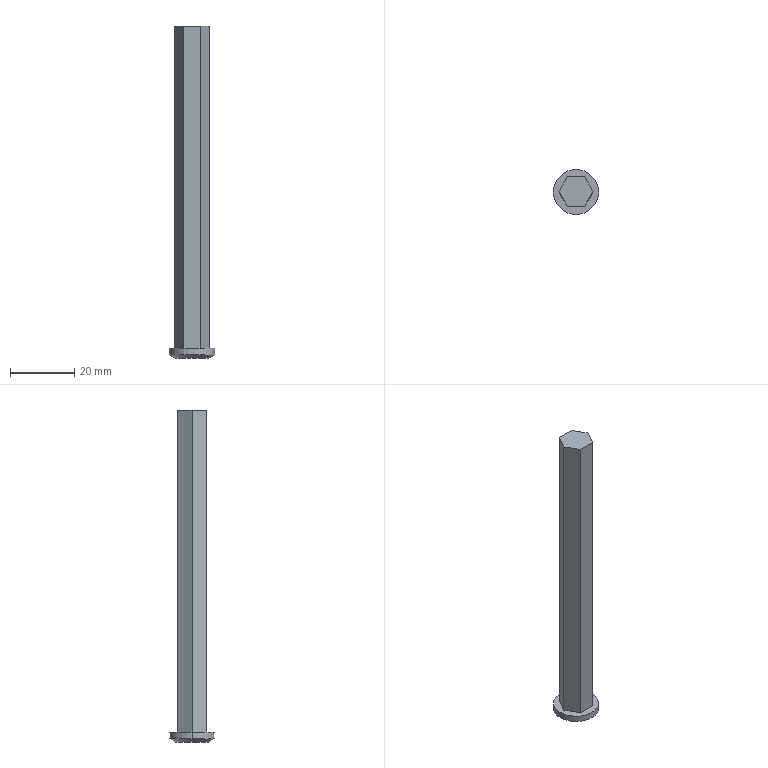Part | SolidWorks | features Chamfer 1, Extrusion 1, ICE 1 | 1 solid | 13 faces | box 14 x 14 x 103 mm | volume 7725 mm3 | plane 9 | cone 2 | cylinder 2 | commonest cylinder face diameters 14 x2
STEP:
#1=CARTESIAN_POINT('',(-5.268,0.,-3.));
#2=VERTEX_POINT('',#1);
#3=CARTESIAN_POINT('',(5.268,0.,-3.));
#4=VERTEX_POINT('',#3);
#5=CARTESIAN_POINT('',(0.,0.,-3.));
#6=DIRECTION('',(0.,0.,-1.));
#7=DIRECTION('',(-1.,0.,0.));
#8=AXIS2_PLACEMENT_3D('',#5,#6,#7);
#9=CIRCLE('',#8,5.268);
#10=EDGE_CURVE('',#2,#4,#9,.T.);
#11=ORIENTED_EDGE('',*,*,#10,.F.);
#12=CARTESIAN_POINT('',(-7.,0.,-2.));
#13=VERTEX_POINT('',#12);
#14=CARTESIAN_POINT('',(-5.268,0.,-3.));
#15=DIRECTION('',(-0.866,0.,0.5));
#16=VECTOR('',#15,1000.);
#17=LINE('',#14,#16);
#18=EDGE_CURVE('',#2,#13,#17,.T.);
#19=ORIENTED_EDGE('',*,*,#18,.T.);
#20=CARTESIAN_POINT('',(7.,0.,-2.));
#21=VERTEX_POINT('',#20);
#22=CARTESIAN_POINT('',(0.,0.,-2.));
#23=DIRECTION('',(0.,0.,1.));
#24=DIRECTION('',(-1.,0.,0.));
#25=AXIS2_PLACEMENT_3D('',#22,#23,#24);
#26=CIRCLE('',#25,7.);
#27=EDGE_CURVE('',#21,#13,#26,.T.);
#28=ORIENTED_EDGE('',*,*,#27,.F.);
#29=CARTESIAN_POINT('',(5.268,0.,-3.));
#30=DIRECTION('',(0.866,0.,0.5));
#31=VECTOR('',#30,1000.);
#32=LINE('',#29,#31);
#33=EDGE_CURVE('',#4,#21,#32,.T.);
#34=ORIENTED_EDGE('',*,*,#33,.F.);
#35=EDGE_LOOP('',(#11,#19,#28,#34));
#36=FACE_OUTER_BOUND('',#35,.T.);
#37=CARTESIAN_POINT('',(0.,0.,-3.));
#38=DIRECTION('',(0.,0.,1.));
#39=DIRECTION('',(1.,0.,0.));
#40=AXIS2_PLACEMENT_3D('',#37,#38,#39);
#41=CONICAL_SURFACE('',#40,5.268,1.047);
#42=ADVANCED_FACE('',(#36),#41,.T.);
#43=ORIENTED_EDGE('',*,*,#27,.T.);
#44=CARTESIAN_POINT('',(-7.,0.,0.));
#45=VERTEX_POINT('',#44);
#46=CARTESIAN_POINT('',(-7.,0.,-3.));
#47=DIRECTION('',(0.,0.,1.));
#48=VECTOR('',#47,1000.);
#49=LINE('',#46,#48);
#50=EDGE_CURVE('',#13,#45,#49,.T.);
#51=ORIENTED_EDGE('',*,*,#50,.T.);
#52=CARTESIAN_POINT('',(7.,0.,0.));
#53=VERTEX_POINT('',#52);
#54=CARTESIAN_POINT('',(0.,0.,0.));
#55=DIRECTION('',(0.,0.,-1.));
#56=DIRECTION('',(-1.,0.,0.));
#57=AXIS2_PLACEMENT_3D('',#54,#55,#56);
#58=CIRCLE('',#57,7.);
#59=EDGE_CURVE('',#45,#53,#58,.T.);
#60=ORIENTED_EDGE('',*,*,#59,.T.);
#61=CARTESIAN_POINT('',(7.,0.,-3.));
#62=DIRECTION('',(0.,0.,1.));
#63=VECTOR('',#62,1000.);
#64=LINE('',#61,#63);
#65=EDGE_CURVE('',#21,#53,#64,.T.);
#66=ORIENTED_EDGE('',*,*,#65,.F.);
#67=EDGE_LOOP('',(#43,#51,#60,#66));
#68=FACE_OUTER_BOUND('',#67,.T.);
#69=CARTESIAN_POINT('',(0.,0.,-3.));
#70=DIRECTION('',(0.,0.,1.));
#71=DIRECTION('',(1.,0.,0.));
#72=AXIS2_PLACEMENT_3D('',#69,#70,#71);
#73=CYLINDRICAL_SURFACE('',#72,7.);
#74=ADVANCED_FACE('',(#68),#73,.T.);
#75=CARTESIAN_POINT('',(-2.65,-4.59,0.));
#76=VERTEX_POINT('',#75);
#77=CARTESIAN_POINT('',(2.65,-4.59,0.));
#78=VERTEX_POINT('',#77);
#79=CARTESIAN_POINT('',(-2.65,-4.59,0.));
#80=DIRECTION('',(1.,0.,0.));
#81=VECTOR('',#80,1000.);
#82=LINE('',#79,#81);
#83=EDGE_CURVE('',#76,#78,#82,.T.);
#84=ORIENTED_EDGE('',*,*,#83,.T.);
#85=CARTESIAN_POINT('',(2.65,-4.59,100.));
#86=VERTEX_POINT('',#85);
#87=CARTESIAN_POINT('',(2.65,-4.59,100.));
#88=DIRECTION('',(0.,0.,-1.));
#89=VECTOR('',#88,1000.);
#90=LINE('',#87,#89);
#91=EDGE_CURVE('',#86,#78,#90,.T.);
#92=ORIENTED_EDGE('',*,*,#91,.F.);
#93=CARTESIAN_POINT('',(-2.65,-4.59,100.));
#94=VERTEX_POINT('',#93);
#95=CARTESIAN_POINT('',(-2.65,-4.59,100.));
#96=DIRECTION('',(1.,0.,0.));
#97=VECTOR('',#96,1000.);
#98=LINE('',#95,#97);
#99=EDGE_CURVE('',#94,#86,#98,.T.);
#100=ORIENTED_EDGE('',*,*,#99,.F.);
#101=CARTESIAN_POINT('',(-2.65,-4.59,100.));
#102=DIRECTION('',(0.,0.,-1.));
#103=VECTOR('',#102,1000.);
#104=LINE('',#101,#103);
#105=EDGE_CURVE('',#94,#76,#104,.T.);
#106=ORIENTED_EDGE('',*,*,#105,.T.);
#107=EDGE_LOOP('',(#84,#92,#100,#106));
#108=FACE_OUTER_BOUND('',#107,.T.);
#109=CARTESIAN_POINT('',(-2.65,-4.59,100.));
#110=DIRECTION('',(0.,1.,0.));
#111=DIRECTION('',(0.,0.,1.));
#112=AXIS2_PLACEMENT_3D('',#109,#110,#111);
#113=PLANE('',#112);
#114=ADVANCED_FACE('',(#108),#113,.F.);
#115=CARTESIAN_POINT('',(5.3,0.,0.));
#116=VERTEX_POINT('',#115);
#117=CARTESIAN_POINT('',(2.65,-4.59,0.));
#118=DIRECTION('',(0.5,0.866,0.));
#119=VECTOR('',#118,1000.);
#120=LINE('',#117,#119);
#121=EDGE_CURVE('',#78,#116,#120,.T.);
#122=ORIENTED_EDGE('',*,*,#121,.T.);
#123=CARTESIAN_POINT('',(5.3,0.,100.));
#124=VERTEX_POINT('',#123);
#125=CARTESIAN_POINT('',(5.3,0.,100.));
#126=DIRECTION('',(0.,0.,-1.));
#127=VECTOR('',#126,1000.);
#128=LINE('',#125,#127);
#129=EDGE_CURVE('',#124,#116,#128,.T.);
#130=ORIENTED_EDGE('',*,*,#129,.F.);
#131=CARTESIAN_POINT('',(2.65,-4.59,100.));
#132=DIRECTION('',(0.5,0.866,0.));
#133=VECTOR('',#132,1000.);
#134=LINE('',#131,#133);
#135=EDGE_CURVE('',#86,#124,#134,.T.);
#136=ORIENTED_EDGE('',*,*,#135,.F.);
#137=ORIENTED_EDGE('',*,*,#91,.T.);
#138=EDGE_LOOP('',(#122,#130,#136,#137));
#139=FACE_OUTER_BOUND('',#138,.T.);
#140=CARTESIAN_POINT('',(2.65,-4.59,100.));
#141=DIRECTION('',(-0.866,0.5,0.));
#142=DIRECTION('',(-0.5,-0.866,0.));
#143=AXIS2_PLACEMENT_3D('',#140,#141,#142);
#144=PLANE('',#143);
#145=ADVANCED_FACE('',(#139),#144,.F.);
#146=CARTESIAN_POINT('',(2.65,4.59,0.));
#147=VERTEX_POINT('',#146);
#148=CARTESIAN_POINT('',(5.3,0.,0.));
#149=DIRECTION('',(-0.5,0.866,0.));
#150=VECTOR('',#149,1000.);
#151=LINE('',#148,#150);
#152=EDGE_CURVE('',#116,#147,#151,.T.);
#153=ORIENTED_EDGE('',*,*,#152,.T.);
#154=CARTESIAN_POINT('',(2.65,4.59,100.));
#155=VERTEX_POINT('',#154);
#156=CARTESIAN_POINT('',(2.65,4.59,100.));
#157=DIRECTION('',(0.,0.,-1.));
#158=VECTOR('',#157,1000.);
#159=LINE('',#156,#158);
#160=EDGE_CURVE('',#155,#147,#159,.T.);
#161=ORIENTED_EDGE('',*,*,#160,.F.);
#162=CARTESIAN_POINT('',(5.3,0.,100.));
#163=DIRECTION('',(-0.5,0.866,0.));
#164=VECTOR('',#163,1000.);
#165=LINE('',#162,#164);
#166=EDGE_CURVE('',#124,#155,#165,.T.);
#167=ORIENTED_EDGE('',*,*,#166,.F.);
#168=ORIENTED_EDGE('',*,*,#129,.T.);
#169=EDGE_LOOP('',(#153,#161,#167,#168));
#170=FACE_OUTER_BOUND('',#169,.T.);
#171=CARTESIAN_POINT('',(5.3,0.,100.));
#172=DIRECTION('',(-0.866,-0.5,0.));
#173=DIRECTION('',(0.5,-0.866,0.));
#174=AXIS2_PLACEMENT_3D('',#171,#172,#173);
#175=PLANE('',#174);
#176=ADVANCED_FACE('',(#170),#175,.F.);
#177=CARTESIAN_POINT('',(-2.65,4.59,0.));
#178=VERTEX_POINT('',#177);
#179=CARTESIAN_POINT('',(2.65,4.59,0.));
#180=DIRECTION('',(-1.,0.,0.));
#181=VECTOR('',#180,1000.);
#182=LINE('',#179,#181);
#183=EDGE_CURVE('',#147,#178,#182,.T.);
#184=ORIENTED_EDGE('',*,*,#183,.T.);
#185=CARTESIAN_POINT('',(-2.65,4.59,100.));
#186=VERTEX_POINT('',#185);
#187=CARTESIAN_POINT('',(-2.65,4.59,100.));
#188=DIRECTION('',(0.,0.,-1.));
#189=VECTOR('',#188,1000.);
#190=LINE('',#187,#189);
#191=EDGE_CURVE('',#186,#178,#190,.T.);
#192=ORIENTED_EDGE('',*,*,#191,.F.);
#193=CARTESIAN_POINT('',(2.65,4.59,100.));
#194=DIRECTION('',(-1.,0.,0.));
#195=VECTOR('',#194,1000.);
#196=LINE('',#193,#195);
#197=EDGE_CURVE('',#155,#186,#196,.T.);
#198=ORIENTED_EDGE('',*,*,#197,.F.);
#199=ORIENTED_EDGE('',*,*,#160,.T.);
#200=EDGE_LOOP('',(#184,#192,#198,#199));
#201=FACE_OUTER_BOUND('',#200,.T.);
#202=CARTESIAN_POINT('',(2.65,4.59,100.));
#203=DIRECTION('',(0.,-1.,0.));
#204=DIRECTION('',(1.,0.,0.));
#205=AXIS2_PLACEMENT_3D('',#202,#203,#204);
#206=PLANE('',#205);
#207=ADVANCED_FACE('',(#201),#206,.F.);
#208=CARTESIAN_POINT('',(-5.3,0.,0.));
#209=VERTEX_POINT('',#208);
#210=CARTESIAN_POINT('',(-2.65,4.59,0.));
#211=DIRECTION('',(-0.5,-0.866,0.));
#212=VECTOR('',#211,1000.);
#213=LINE('',#210,#212);
#214=EDGE_CURVE('',#178,#209,#213,.T.);
#215=ORIENTED_EDGE('',*,*,#214,.T.);
#216=CARTESIAN_POINT('',(-5.3,0.,100.));
#217=VERTEX_POINT('',#216);
#218=CARTESIAN_POINT('',(-5.3,0.,100.));
#219=DIRECTION('',(0.,0.,-1.));
#220=VECTOR('',#219,1000.);
#221=LINE('',#218,#220);
#222=EDGE_CURVE('',#217,#209,#221,.T.);
#223=ORIENTED_EDGE('',*,*,#222,.F.);
#224=CARTESIAN_POINT('',(-2.65,4.59,100.));
#225=DIRECTION('',(-0.5,-0.866,0.));
#226=VECTOR('',#225,1000.);
#227=LINE('',#224,#226);
#228=EDGE_CURVE('',#186,#217,#227,.T.);
#229=ORIENTED_EDGE('',*,*,#228,.F.);
#230=ORIENTED_EDGE('',*,*,#191,.T.);
#231=EDGE_LOOP('',(#215,#223,#229,#230));
#232=FACE_OUTER_BOUND('',#231,.T.);
#233=CARTESIAN_POINT('',(-2.65,4.59,100.));
#234=DIRECTION('',(0.866,-0.5,0.));
#235=DIRECTION('',(0.5,0.866,0.));
#236=AXIS2_PLACEMENT_3D('',#233,#234,#235);
#237=PLANE('',#236);
#238=ADVANCED_FACE('',(#232),#237,.F.);
#239=CARTESIAN_POINT('',(-5.3,0.,0.));
#240=DIRECTION('',(0.5,-0.866,0.));
#241=VECTOR('',#240,1000.);
#242=LINE('',#239,#241);
#243=EDGE_CURVE('',#209,#76,#242,.T.);
#244=ORIENTED_EDGE('',*,*,#243,.T.);
#245=ORIENTED_EDGE('',*,*,#105,.F.);
#246=CARTESIAN_POINT('',(-5.3,0.,100.));
#247=DIRECTION('',(0.5,-0.866,0.));
#248=VECTOR('',#247,1000.);
#249=LINE('',#246,#248);
#250=EDGE_CURVE('',#217,#94,#249,.T.);
#251=ORIENTED_EDGE('',*,*,#250,.F.);
#252=ORIENTED_EDGE('',*,*,#222,.T.);
#253=EDGE_LOOP('',(#244,#245,#251,#252));
#254=FACE_OUTER_BOUND('',#253,.T.);
#255=CARTESIAN_POINT('',(-5.3,0.,100.));
#256=DIRECTION('',(0.866,0.5,0.));
#257=DIRECTION('',(-0.5,0.866,0.));
#258=AXIS2_PLACEMENT_3D('',#255,#256,#257);
#259=PLANE('',#258);
#260=ADVANCED_FACE('',(#254),#259,.F.);
#261=ORIENTED_EDGE('',*,*,#99,.T.);
#262=ORIENTED_EDGE('',*,*,#135,.T.);
#263=ORIENTED_EDGE('',*,*,#166,.T.);
#264=ORIENTED_EDGE('',*,*,#197,.T.);
#265=ORIENTED_EDGE('',*,*,#228,.T.);
#266=ORIENTED_EDGE('',*,*,#250,.T.);
#267=EDGE_LOOP('',(#261,#262,#263,#264,#265,#266));
#268=FACE_OUTER_BOUND('',#267,.T.);
#269=CARTESIAN_POINT('',(0.,0.,100.));
#270=DIRECTION('',(0.,0.,1.));
#271=DIRECTION('',(1.,0.,0.));
#272=AXIS2_PLACEMENT_3D('',#269,#270,#271);
#273=PLANE('',#272);
#274=ADVANCED_FACE('',(#268),#273,.T.);
#275=ORIENTED_EDGE('',*,*,#50,.F.);
#276=CARTESIAN_POINT('',(0.,0.,-2.));
#277=DIRECTION('',(0.,0.,1.));
#278=DIRECTION('',(-1.,0.,0.));
#279=AXIS2_PLACEMENT_3D('',#276,#277,#278);
#280=CIRCLE('',#279,7.);
#281=EDGE_CURVE('',#13,#21,#280,.T.);
#282=ORIENTED_EDGE('',*,*,#281,.T.);
#283=ORIENTED_EDGE('',*,*,#65,.T.);
#284=CARTESIAN_POINT('',(0.,0.,0.));
#285=DIRECTION('',(0.,0.,-1.));
#286=DIRECTION('',(-1.,0.,0.));
#287=AXIS2_PLACEMENT_3D('',#284,#285,#286);
#288=CIRCLE('',#287,7.);
#289=EDGE_CURVE('',#53,#45,#288,.T.);
#290=ORIENTED_EDGE('',*,*,#289,.T.);
#291=EDGE_LOOP('',(#275,#282,#283,#290));
#292=FACE_OUTER_BOUND('',#291,.T.);
#293=CARTESIAN_POINT('',(0.,0.,-3.));
#294=DIRECTION('',(0.,0.,1.));
#295=DIRECTION('',(1.,0.,0.));
#296=AXIS2_PLACEMENT_3D('',#293,#294,#295);
#297=CYLINDRICAL_SURFACE('',#296,7.);
#298=ADVANCED_FACE('',(#292),#297,.T.);
#299=CARTESIAN_POINT('',(0.,0.,-3.));
#300=DIRECTION('',(0.,0.,-1.));
#301=DIRECTION('',(-1.,0.,0.));
#302=AXIS2_PLACEMENT_3D('',#299,#300,#301);
#303=CIRCLE('',#302,5.268);
#304=EDGE_CURVE('',#4,#2,#303,.T.);
#305=ORIENTED_EDGE('',*,*,#304,.T.);
#306=ORIENTED_EDGE('',*,*,#10,.T.);
#307=EDGE_LOOP('',(#305,#306));
#308=FACE_OUTER_BOUND('',#307,.T.);
#309=CARTESIAN_POINT('',(0.,0.,-3.));
#310=DIRECTION('',(0.,0.,-1.));
#311=DIRECTION('',(-1.,0.,0.));
#312=AXIS2_PLACEMENT_3D('',#309,#310,#311);
#313=PLANE('',#312);
#314=ADVANCED_FACE('',(#308),#313,.T.);
#315=ORIENTED_EDGE('',*,*,#83,.F.);
#316=ORIENTED_EDGE('',*,*,#243,.F.);
#317=ORIENTED_EDGE('',*,*,#214,.F.);
#318=ORIENTED_EDGE('',*,*,#183,.F.);
#319=ORIENTED_EDGE('',*,*,#152,.F.);
#320=ORIENTED_EDGE('',*,*,#121,.F.);
#321=EDGE_LOOP('',(#315,#316,#317,#318,#319,#320));
#322=FACE_BOUND('',#321,.T.);
#323=ORIENTED_EDGE('',*,*,#289,.F.);
#324=ORIENTED_EDGE('',*,*,#59,.F.);
#325=EDGE_LOOP('',(#323,#324));
#326=FACE_OUTER_BOUND('',#325,.T.);
#327=CARTESIAN_POINT('',(0.,0.,0.));
#328=DIRECTION('',(0.,0.,-1.));
#329=DIRECTION('',(-1.,0.,0.));
#330=AXIS2_PLACEMENT_3D('',#327,#328,#329);
#331=PLANE('',#330);
#332=ADVANCED_FACE('',(#322,#326),#331,.F.);
#333=ORIENTED_EDGE('',*,*,#18,.F.);
#334=ORIENTED_EDGE('',*,*,#304,.F.);
#335=ORIENTED_EDGE('',*,*,#33,.T.);
#336=ORIENTED_EDGE('',*,*,#281,.F.);
#337=EDGE_LOOP('',(#333,#334,#335,#336));
#338=FACE_OUTER_BOUND('',#337,.T.);
#339=CARTESIAN_POINT('',(0.,0.,-3.));
#340=DIRECTION('',(0.,0.,1.));
#341=DIRECTION('',(1.,0.,0.));
#342=AXIS2_PLACEMENT_3D('',#339,#340,#341);
#343=CONICAL_SURFACE('',#342,5.268,1.047);
#344=ADVANCED_FACE('',(#338),#343,.T.);
#345=CLOSED_SHELL('',(#42,#74,#114,#145,#176,#207,#238,#260,#274,#298,#314,#332,#344));
#346=MANIFOLD_SOLID_BREP('',#345);
#347=CARTESIAN_POINT('',(0.,0.,0.));
#348=DIRECTION('',(0.,0.,1.));
#349=DIRECTION('',(1.,0.,0.));
#350=AXIS2_PLACEMENT_3D('',#347,#348,#349);
#351=(LENGTH_UNIT()NAMED_UNIT(*)SI_UNIT(.MILLI.,.METRE.));
#352=UNCERTAINTY_MEASURE_WITH_UNIT(LENGTH_MEASURE(0.00001),#351,'','');
#353=(NAMED_UNIT(*)PLANE_ANGLE_UNIT()SI_UNIT($,.RADIAN.));
#354=(NAMED_UNIT(*)SI_UNIT($,.STERADIAN.)SOLID_ANGLE_UNIT());
#355=(GEOMETRIC_REPRESENTATION_CONTEXT(3)GLOBAL_UNCERTAINTY_ASSIGNED_CONTEXT((#352))GLOBAL_UNIT_ASSIGNED_CONTEXT((#351,#353,#354))REPRESENTATION_CONTEXT('',''));
#356=ADVANCED_BREP_SHAPE_REPRESENTATION('',(#346,#350),#355);